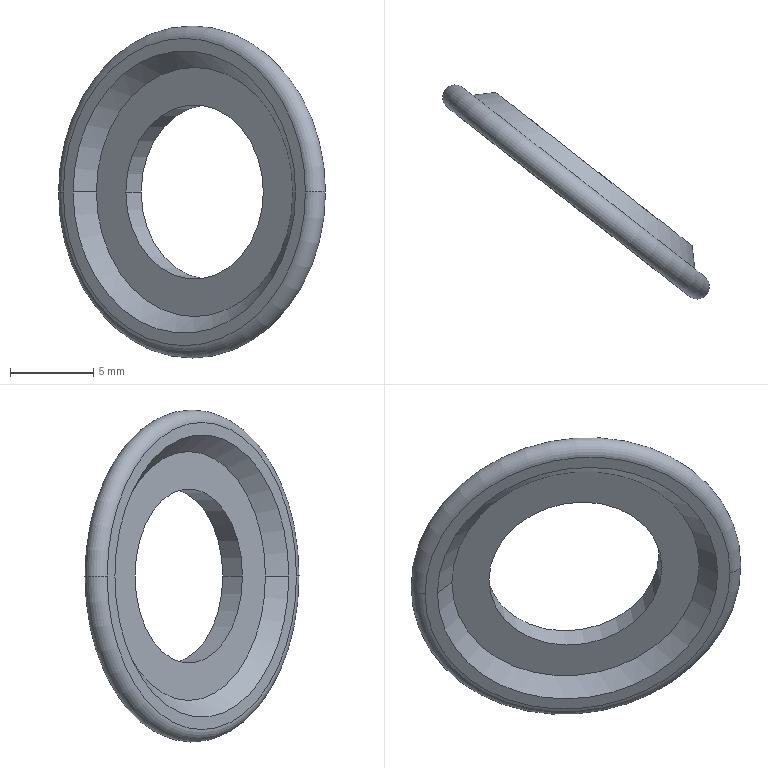Part | STEP file | VALVE_3PARTV11 | 1 solid | 12 faces | box 16.078 x 12.89 x 20 mm | volume 326.438 mm3 | cone 4 | plane 4 | torus 2 | cylinder 2 | commonest cylinder face diameters 10.5 x2
STEP:
#1=CARTESIAN_POINT('',(0.,0.,0.));
#2=DIRECTION('',(0.,0.,1.));
#3=DIRECTION('',(1.,0.,0.));
#4=AXIS2_PLACEMENT_3D('',#1,#2,#3);
#5=CARTESIAN_POINT('',(-0.6961,8.953,0.));
#6=VERTEX_POINT('',#5);
#7=CARTESIAN_POINT('',(13.882,-2.437,0.));
#8=VERTEX_POINT('',#7);
#9=CARTESIAN_POINT('',(6.593,3.258,0.));
#10=DIRECTION('',(0.6157,0.788,0.));
#11=DIRECTION('',(-0.788,0.6157,0.));
#12=AXIS2_PLACEMENT_3D('',#9,#10,#11);
#13=CIRCLE('',#12,9.25);
#14=CARTESIAN_POINT('',(7.055,3.849,0.));
#15=DIRECTION('',(0.6157,0.788,0.));
#16=DIRECTION('',(-0.788,0.6157,0.));
#17=AXIS2_PLACEMENT_3D('',#14,#15,#16);
#18=TOROIDAL_SURFACE('',#17,9.25,0.75);
#19=CARTESIAN_POINT('',(0.,-1.571));
#20=DIRECTION('',(1.,0.));
#21=VECTOR('',#20,1.);
#22=LINE('',#19,#21);
#23=(GEOMETRIC_REPRESENTATION_CONTEXT(2)PARAMETRIC_REPRESENTATION_CONTEXT()REPRESENTATION_CONTEXT('',''));
#24=DEFINITIONAL_REPRESENTATION('',(#22),#23);
#25=PCURVE('',#18,#24);
#26=CARTESIAN_POINT('',(-0.6961,8.953,0.));
#27=DIRECTION('',(-0.6157,-0.788,0.));
#28=DIRECTION('',(0.788,-0.6157,0.));
#29=AXIS2_PLACEMENT_3D('',#26,#27,#28);
#30=PLANE('',#29);
#31=CARTESIAN_POINT('',(0.,0.));
#32=CARTESIAN_POINT('',(0.,16.021));
#33=CARTESIAN_POINT('',(13.875,8.011));
#34=CARTESIAN_POINT('',(27.75,0.));
#35=CARTESIAN_POINT('',(13.875,-8.011));
#36=CARTESIAN_POINT('',(0.,-16.021));
#37=CARTESIAN_POINT('',(0.,0.));
#38=(BOUNDED_CURVE()B_SPLINE_CURVE(2,(#31,#32,#33,#34,#35,#36,#37),.UNSPECIFIED.,.T.,.F.)B_SPLINE_CURVE_WITH_KNOTS((1,2,2,2,2,1),(-2.094,0.,2.094,4.189,6.283,8.378),.UNSPECIFIED.)CURVE()GEOMETRIC_REPRESENTATION_ITEM()RATIONAL_B_SPLINE_CURVE((1.,0.5,1.,0.5,1.,0.5,1.))REPRESENTATION_ITEM(''));
#39=(GEOMETRIC_REPRESENTATION_CONTEXT(2)PARAMETRIC_REPRESENTATION_CONTEXT()REPRESENTATION_CONTEXT('',''));
#40=DEFINITIONAL_REPRESENTATION('',(#38),#39);
#41=PCURVE('',#30,#40);
#42=SURFACE_CURVE('',#13,(#25,#41),.PCURVE_S1.);
#43=EDGE_CURVE('',#6,#8,#42,.T.);
#44=ORIENTED_EDGE('',*,*,#43,.T.);
#45=CARTESIAN_POINT('',(14.806,-1.255,0.));
#46=VERTEX_POINT('',#45);
#47=CARTESIAN_POINT('',(14.344,-1.846,0.));
#48=DIRECTION('',(0.,0.,1.));
#49=DIRECTION('',(1.,0.,0.));
#50=AXIS2_PLACEMENT_3D('',#47,#48,#49);
#51=CIRCLE('',#50,0.75);
#52=CARTESIAN_POINT('',(3.142,-5.62));
#53=DIRECTION('',(0.,1.));
#54=VECTOR('',#53,1.);
#55=LINE('',#52,#54);
#56=(GEOMETRIC_REPRESENTATION_CONTEXT(2)PARAMETRIC_REPRESENTATION_CONTEXT()REPRESENTATION_CONTEXT('',''));
#57=DEFINITIONAL_REPRESENTATION('',(#55),#56);
#58=PCURVE('',#18,#57);
#59=CARTESIAN_POINT('',(7.055,3.849,0.));
#60=DIRECTION('',(0.6157,0.788,0.));
#61=DIRECTION('',(-0.788,0.6157,0.));
#62=AXIS2_PLACEMENT_3D('',#59,#60,#61);
#63=TOROIDAL_SURFACE('',#62,9.25,0.75);
#64=CARTESIAN_POINT('',(3.142,-5.62));
#65=DIRECTION('',(0.,1.));
#66=VECTOR('',#65,1.);
#67=LINE('',#64,#66);
#68=(GEOMETRIC_REPRESENTATION_CONTEXT(2)PARAMETRIC_REPRESENTATION_CONTEXT()REPRESENTATION_CONTEXT('',''));
#69=DEFINITIONAL_REPRESENTATION('',(#67),#68);
#70=PCURVE('',#63,#69);
#71=SURFACE_CURVE('',#51,(#58,#70),.PCURVE_S1.);
#72=EDGE_CURVE('',#8,#46,#71,.T.);
#73=ORIENTED_EDGE('',*,*,#72,.T.);
#74=CARTESIAN_POINT('',(0.2274,10.135,0.));
#75=VERTEX_POINT('',#74);
#76=CARTESIAN_POINT('',(7.517,4.44,0.));
#77=DIRECTION('',(0.6157,0.788,0.));
#78=DIRECTION('',(-0.788,0.6157,0.));
#79=AXIS2_PLACEMENT_3D('',#76,#77,#78);
#80=CIRCLE('',#79,9.25);
#81=CARTESIAN_POINT('',(0.,1.571));
#82=DIRECTION('',(1.,0.));
#83=VECTOR('',#82,1.);
#84=LINE('',#81,#83);
#85=(GEOMETRIC_REPRESENTATION_CONTEXT(2)PARAMETRIC_REPRESENTATION_CONTEXT()REPRESENTATION_CONTEXT('',''));
#86=DEFINITIONAL_REPRESENTATION('',(#84),#85);
#87=PCURVE('',#18,#86);
#88=CARTESIAN_POINT('',(0.8184,9.673,0.));
#89=DIRECTION('',(0.6157,0.788,0.));
#90=DIRECTION('',(-0.788,0.6157,0.));
#91=AXIS2_PLACEMENT_3D('',#88,#89,#90);
#92=PLANE('',#91);
#93=CARTESIAN_POINT('',(-8.5,0.));
#94=DIRECTION('',(1.,0.));
#95=AXIS2_PLACEMENT_2D('',#93,#94);
#96=CIRCLE('',#95,9.25);
#97=(GEOMETRIC_REPRESENTATION_CONTEXT(2)PARAMETRIC_REPRESENTATION_CONTEXT()REPRESENTATION_CONTEXT('',''));
#98=DEFINITIONAL_REPRESENTATION('',(#96),#97);
#99=PCURVE('',#92,#98);
#100=SURFACE_CURVE('',#80,(#87,#99),.PCURVE_S1.);
#101=EDGE_CURVE('',#75,#46,#100,.T.);
#102=ORIENTED_EDGE('',*,*,#101,.F.);
#103=CARTESIAN_POINT('',(-0.2343,9.544,0.));
#104=DIRECTION('',(0.,0.,-1.));
#105=DIRECTION('',(-1.,0.,0.));
#106=AXIS2_PLACEMENT_3D('',#103,#104,#105);
#107=CIRCLE('',#106,0.75);
#108=CARTESIAN_POINT('',(0.,-6.946));
#109=DIRECTION('',(0.,1.));
#110=VECTOR('',#109,1.);
#111=LINE('',#108,#110);
#112=(GEOMETRIC_REPRESENTATION_CONTEXT(2)PARAMETRIC_REPRESENTATION_CONTEXT()REPRESENTATION_CONTEXT('',''));
#113=DEFINITIONAL_REPRESENTATION('',(#111),#112);
#114=PCURVE('',#18,#113);
#115=CARTESIAN_POINT('',(6.283,-6.946));
#116=DIRECTION('',(0.,1.));
#117=VECTOR('',#116,1.);
#118=LINE('',#115,#117);
#119=(GEOMETRIC_REPRESENTATION_CONTEXT(2)PARAMETRIC_REPRESENTATION_CONTEXT()REPRESENTATION_CONTEXT('',''));
#120=DEFINITIONAL_REPRESENTATION('',(#118),#119);
#121=PCURVE('',#63,#120);
#122=SURFACE_CURVE('',#107,(#114,#121),.PCURVE_S1.);
#123=EDGE_CURVE('',#6,#75,#122,.T.);
#124=ORIENTED_EDGE('',*,*,#123,.F.);
#125=EDGE_LOOP('',(#44,#73,#102,#124));
#126=FACE_BOUND('',#125,.T.);
#127=ADVANCED_FACE('',(#126),#18,.T.);
#128=CARTESIAN_POINT('',(2.222,9.846,0.));
#129=VERTEX_POINT('',#128);
#130=CARTESIAN_POINT('',(14.042,0.6108,0.));
#131=VERTEX_POINT('',#130);
#132=CARTESIAN_POINT('',(8.132,5.228,0.));
#133=DIRECTION('',(0.6157,0.788,0.));
#134=DIRECTION('',(-0.788,0.6157,0.));
#135=AXIS2_PLACEMENT_3D('',#132,#133,#134);
#136=CIRCLE('',#135,7.5);
#137=CARTESIAN_POINT('',(8.132,5.228,0.));
#138=DIRECTION('',(-0.6157,-0.788,0.));
#139=DIRECTION('',(0.788,-0.6157,0.));
#140=AXIS2_PLACEMENT_3D('',#137,#138,#139);
#141=CONICAL_SURFACE('',#140,7.5,0.7854);
#142=CARTESIAN_POINT('',(3.142,0.));
#143=DIRECTION('',(-1.,0.));
#144=VECTOR('',#143,1.);
#145=LINE('',#142,#144);
#146=(GEOMETRIC_REPRESENTATION_CONTEXT(2)PARAMETRIC_REPRESENTATION_CONTEXT()REPRESENTATION_CONTEXT('',''));
#147=DEFINITIONAL_REPRESENTATION('',(#145),#146);
#148=PCURVE('',#141,#147);
#149=CARTESIAN_POINT('',(3.995,8.46,0.));
#150=DIRECTION('',(0.6157,0.788,0.));
#151=DIRECTION('',(-0.788,0.6157,0.));
#152=AXIS2_PLACEMENT_3D('',#149,#150,#151);
#153=PLANE('',#152);
#154=CARTESIAN_POINT('',(-5.25,0.));
#155=DIRECTION('',(1.,0.));
#156=AXIS2_PLACEMENT_2D('',#154,#155);
#157=CIRCLE('',#156,7.5);
#158=(GEOMETRIC_REPRESENTATION_CONTEXT(2)PARAMETRIC_REPRESENTATION_CONTEXT()REPRESENTATION_CONTEXT('',''));
#159=DEFINITIONAL_REPRESENTATION('',(#157),#158);
#160=PCURVE('',#153,#159);
#161=SURFACE_CURVE('',#136,(#148,#160),.PCURVE_S1.);
#162=EDGE_CURVE('',#129,#131,#161,.T.);
#163=ORIENTED_EDGE('',*,*,#162,.F.);
#164=CARTESIAN_POINT('',(0.8184,9.673,0.));
#165=VERTEX_POINT('',#164);
#166=CARTESIAN_POINT('',(2.222,9.846,0.));
#167=DIRECTION('',(-0.9925,-0.1219,0.));
#168=VECTOR('',#167,1.);
#169=LINE('',#166,#168);
#170=CARTESIAN_POINT('',(3.142,0.));
#171=DIRECTION('',(0.,1.));
#172=VECTOR('',#171,1.);
#173=LINE('',#170,#172);
#174=(GEOMETRIC_REPRESENTATION_CONTEXT(2)PARAMETRIC_REPRESENTATION_CONTEXT()REPRESENTATION_CONTEXT('',''));
#175=DEFINITIONAL_REPRESENTATION('',(#173),#174);
#176=PCURVE('',#141,#175);
#177=CARTESIAN_POINT('',(8.132,5.228,0.));
#178=DIRECTION('',(-0.6157,-0.788,0.));
#179=DIRECTION('',(0.788,-0.6157,0.));
#180=AXIS2_PLACEMENT_3D('',#177,#178,#179);
#181=CONICAL_SURFACE('',#180,7.5,0.7854);
#182=CARTESIAN_POINT('',(3.142,0.));
#183=DIRECTION('',(0.,1.));
#184=VECTOR('',#183,1.);
#185=LINE('',#182,#184);
#186=(GEOMETRIC_REPRESENTATION_CONTEXT(2)PARAMETRIC_REPRESENTATION_CONTEXT()REPRESENTATION_CONTEXT('',''));
#187=DEFINITIONAL_REPRESENTATION('',(#185),#186);
#188=PCURVE('',#181,#187);
#189=SURFACE_CURVE('',#169,(#176,#188),.PCURVE_S1.);
#190=EDGE_CURVE('',#129,#165,#189,.T.);
#191=ORIENTED_EDGE('',*,*,#190,.T.);
#192=CARTESIAN_POINT('',(14.215,-0.7929,0.));
#193=VERTEX_POINT('',#192);
#194=CARTESIAN_POINT('',(7.517,4.44,0.));
#195=DIRECTION('',(0.6157,0.788,0.));
#196=DIRECTION('',(-0.788,0.6157,0.));
#197=AXIS2_PLACEMENT_3D('',#194,#195,#196);
#198=CIRCLE('',#197,8.5);
#199=CARTESIAN_POINT('',(3.142,1.));
#200=DIRECTION('',(-1.,0.));
#201=VECTOR('',#200,1.);
#202=LINE('',#199,#201);
#203=(GEOMETRIC_REPRESENTATION_CONTEXT(2)PARAMETRIC_REPRESENTATION_CONTEXT()REPRESENTATION_CONTEXT('',''));
#204=DEFINITIONAL_REPRESENTATION('',(#202),#203);
#205=PCURVE('',#141,#204);
#206=CARTESIAN_POINT('',(-8.5,0.));
#207=DIRECTION('',(1.,0.));
#208=AXIS2_PLACEMENT_2D('',#206,#207);
#209=CIRCLE('',#208,8.5);
#210=(GEOMETRIC_REPRESENTATION_CONTEXT(2)PARAMETRIC_REPRESENTATION_CONTEXT()REPRESENTATION_CONTEXT('',''));
#211=DEFINITIONAL_REPRESENTATION('',(#209),#210);
#212=PCURVE('',#92,#211);
#213=SURFACE_CURVE('',#198,(#205,#212),.PCURVE_S1.);
#214=EDGE_CURVE('',#165,#193,#213,.T.);
#215=ORIENTED_EDGE('',*,*,#214,.T.);
#216=CARTESIAN_POINT('',(14.042,0.6108,0.));
#217=DIRECTION('',(0.1219,-0.9925,0.));
#218=VECTOR('',#217,1.);
#219=LINE('',#216,#218);
#220=CARTESIAN_POINT('',(0.,0.));
#221=DIRECTION('',(0.,1.));
#222=VECTOR('',#221,1.);
#223=LINE('',#220,#222);
#224=(GEOMETRIC_REPRESENTATION_CONTEXT(2)PARAMETRIC_REPRESENTATION_CONTEXT()REPRESENTATION_CONTEXT('',''));
#225=DEFINITIONAL_REPRESENTATION('',(#223),#224);
#226=PCURVE('',#141,#225);
#227=CARTESIAN_POINT('',(6.283,0.));
#228=DIRECTION('',(0.,1.));
#229=VECTOR('',#228,1.);
#230=LINE('',#227,#229);
#231=(GEOMETRIC_REPRESENTATION_CONTEXT(2)PARAMETRIC_REPRESENTATION_CONTEXT()REPRESENTATION_CONTEXT('',''));
#232=DEFINITIONAL_REPRESENTATION('',(#230),#231);
#233=PCURVE('',#181,#232);
#234=SURFACE_CURVE('',#219,(#226,#233),.PCURVE_S1.);
#235=EDGE_CURVE('',#131,#193,#234,.T.);
#236=ORIENTED_EDGE('',*,*,#235,.F.);
#237=EDGE_LOOP('',(#163,#191,#215,#236));
#238=FACE_BOUND('',#237,.T.);
#239=ADVANCED_FACE('',(#238),#141,.T.);
#240=CARTESIAN_POINT('',(3.072,7.278,0.));
#241=VERTEX_POINT('',#240);
#242=CARTESIAN_POINT('',(3.995,8.46,0.));
#243=VERTEX_POINT('',#242);
#244=CARTESIAN_POINT('',(-6.471,-4.936,0.));
#245=DIRECTION('',(0.6157,0.788,0.));
#246=VECTOR('',#245,1.);
#247=LINE('',#244,#246);
#248=CARTESIAN_POINT('',(-2.334,-8.168,0.));
#249=DIRECTION('',(0.6157,0.788,0.));
#250=DIRECTION('',(-0.788,0.6157,0.));
#251=AXIS2_PLACEMENT_3D('',#248,#249,#250);
#252=CYLINDRICAL_SURFACE('',#251,5.25);
#253=CARTESIAN_POINT('',(6.283,0.));
#254=DIRECTION('',(0.,1.));
#255=VECTOR('',#254,1.);
#256=LINE('',#253,#255);
#257=(GEOMETRIC_REPRESENTATION_CONTEXT(2)PARAMETRIC_REPRESENTATION_CONTEXT()REPRESENTATION_CONTEXT('',''));
#258=DEFINITIONAL_REPRESENTATION('',(#256),#257);
#259=PCURVE('',#252,#258);
#260=CARTESIAN_POINT('',(-2.334,-8.168,0.));
#261=DIRECTION('',(0.6157,0.788,0.));
#262=DIRECTION('',(-0.788,0.6157,0.));
#263=AXIS2_PLACEMENT_3D('',#260,#261,#262);
#264=CYLINDRICAL_SURFACE('',#263,5.25);
#265=CARTESIAN_POINT('',(0.,0.));
#266=DIRECTION('',(0.,1.));
#267=VECTOR('',#266,1.);
#268=LINE('',#265,#267);
#269=(GEOMETRIC_REPRESENTATION_CONTEXT(2)PARAMETRIC_REPRESENTATION_CONTEXT()REPRESENTATION_CONTEXT('',''));
#270=DEFINITIONAL_REPRESENTATION('',(#268),#269);
#271=PCURVE('',#264,#270);
#272=SURFACE_CURVE('',#247,(#259,#271),.PCURVE_S1.);
#273=EDGE_CURVE('',#241,#243,#272,.T.);
#274=ORIENTED_EDGE('',*,*,#273,.T.);
#275=CARTESIAN_POINT('',(12.269,1.996,0.));
#276=VERTEX_POINT('',#275);
#277=CARTESIAN_POINT('',(8.132,5.228,0.));
#278=DIRECTION('',(0.6157,0.788,0.));
#279=DIRECTION('',(-0.788,0.6157,0.));
#280=AXIS2_PLACEMENT_3D('',#277,#278,#279);
#281=CIRCLE('',#280,5.25);
#282=CARTESIAN_POINT('',(0.,17.));
#283=DIRECTION('',(1.,0.));
#284=VECTOR('',#283,1.);
#285=LINE('',#282,#284);
#286=(GEOMETRIC_REPRESENTATION_CONTEXT(2)PARAMETRIC_REPRESENTATION_CONTEXT()REPRESENTATION_CONTEXT('',''));
#287=DEFINITIONAL_REPRESENTATION('',(#285),#286);
#288=PCURVE('',#252,#287);
#289=CARTESIAN_POINT('',(-5.25,0.));
#290=DIRECTION('',(1.,0.));
#291=AXIS2_PLACEMENT_2D('',#289,#290);
#292=CIRCLE('',#291,5.25);
#293=(GEOMETRIC_REPRESENTATION_CONTEXT(2)PARAMETRIC_REPRESENTATION_CONTEXT()REPRESENTATION_CONTEXT('',''));
#294=DEFINITIONAL_REPRESENTATION('',(#292),#293);
#295=PCURVE('',#153,#294);
#296=SURFACE_CURVE('',#281,(#288,#295),.PCURVE_S1.);
#297=EDGE_CURVE('',#276,#243,#296,.T.);
#298=ORIENTED_EDGE('',*,*,#297,.F.);
#299=CARTESIAN_POINT('',(11.346,0.814,0.));
#300=VERTEX_POINT('',#299);
#301=CARTESIAN_POINT('',(1.803,-11.4,0.));
#302=DIRECTION('',(0.6157,0.788,0.));
#303=VECTOR('',#302,1.);
#304=LINE('',#301,#303);
#305=CARTESIAN_POINT('',(3.142,0.));
#306=DIRECTION('',(0.,1.));
#307=VECTOR('',#306,1.);
#308=LINE('',#305,#307);
#309=(GEOMETRIC_REPRESENTATION_CONTEXT(2)PARAMETRIC_REPRESENTATION_CONTEXT()REPRESENTATION_CONTEXT('',''));
#310=DEFINITIONAL_REPRESENTATION('',(#308),#309);
#311=PCURVE('',#252,#310);
#312=CARTESIAN_POINT('',(3.142,0.));
#313=DIRECTION('',(0.,1.));
#314=VECTOR('',#313,1.);
#315=LINE('',#312,#314);
#316=(GEOMETRIC_REPRESENTATION_CONTEXT(2)PARAMETRIC_REPRESENTATION_CONTEXT()REPRESENTATION_CONTEXT('',''));
#317=DEFINITIONAL_REPRESENTATION('',(#315),#316);
#318=PCURVE('',#264,#317);
#319=SURFACE_CURVE('',#304,(#311,#318),.PCURVE_S1.);
#320=EDGE_CURVE('',#300,#276,#319,.T.);
#321=ORIENTED_EDGE('',*,*,#320,.F.);
#322=CARTESIAN_POINT('',(7.209,4.046,0.));
#323=DIRECTION('',(0.6157,0.788,0.));
#324=DIRECTION('',(-0.788,0.6157,0.));
#325=AXIS2_PLACEMENT_3D('',#322,#323,#324);
#326=CIRCLE('',#325,5.25);
#327=CARTESIAN_POINT('',(0.,15.5));
#328=DIRECTION('',(1.,0.));
#329=VECTOR('',#328,1.);
#330=LINE('',#327,#329);
#331=(GEOMETRIC_REPRESENTATION_CONTEXT(2)PARAMETRIC_REPRESENTATION_CONTEXT()REPRESENTATION_CONTEXT('',''));
#332=DEFINITIONAL_REPRESENTATION('',(#330),#331);
#333=PCURVE('',#252,#332);
#334=CARTESIAN_POINT('',(1.299,8.664,0.));
#335=DIRECTION('',(-0.6157,-0.788,0.));
#336=DIRECTION('',(0.788,-0.6157,0.));
#337=AXIS2_PLACEMENT_3D('',#334,#335,#336);
#338=PLANE('',#337);
#339=CARTESIAN_POINT('',(2.25,0.));
#340=CARTESIAN_POINT('',(2.25,9.093));
#341=CARTESIAN_POINT('',(10.125,4.547));
#342=CARTESIAN_POINT('',(18.,0.));
#343=CARTESIAN_POINT('',(10.125,-4.547));
#344=CARTESIAN_POINT('',(2.25,-9.093));
#345=CARTESIAN_POINT('',(2.25,0.));
#346=(BOUNDED_CURVE()B_SPLINE_CURVE(2,(#339,#340,#341,#342,#343,#344,#345),.UNSPECIFIED.,.T.,.F.)B_SPLINE_CURVE_WITH_KNOTS((1,2,2,2,2,1),(-2.094,0.,2.094,4.189,6.283,8.378),.UNSPECIFIED.)CURVE()GEOMETRIC_REPRESENTATION_ITEM()RATIONAL_B_SPLINE_CURVE((1.,0.5,1.,0.5,1.,0.5,1.))REPRESENTATION_ITEM(''));
#347=(GEOMETRIC_REPRESENTATION_CONTEXT(2)PARAMETRIC_REPRESENTATION_CONTEXT()REPRESENTATION_CONTEXT('',''));
#348=DEFINITIONAL_REPRESENTATION('',(#346),#347);
#349=PCURVE('',#338,#348);
#350=SURFACE_CURVE('',#326,(#333,#349),.PCURVE_S1.);
#351=EDGE_CURVE('',#300,#241,#350,.T.);
#352=ORIENTED_EDGE('',*,*,#351,.T.);
#353=EDGE_LOOP('',(#274,#298,#321,#352));
#354=FACE_BOUND('',#353,.F.);
#355=ADVANCED_FACE('',(#354),#252,.F.);
#356=CARTESIAN_POINT('',(13.119,-0.5713,0.));
#357=VERTEX_POINT('',#356);
#358=CARTESIAN_POINT('',(13.291,-1.975,0.));
#359=VERTEX_POINT('',#358);
#360=CARTESIAN_POINT('',(13.291,-1.975,0.));
#361=DIRECTION('',(0.1219,-0.9925,0.));
#362=VECTOR('',#361,1.);
#363=LINE('',#360,#362);
#364=CARTESIAN_POINT('',(6.593,3.258,0.));
#365=DIRECTION('',(-0.6157,-0.788,0.));
#366=DIRECTION('',(0.788,-0.6157,0.));
#367=AXIS2_PLACEMENT_3D('',#364,#365,#366);
#368=CONICAL_SURFACE('',#367,8.5,0.7854);
#369=CARTESIAN_POINT('',(6.283,0.));
#370=DIRECTION('',(0.,1.));
#371=VECTOR('',#370,1.);
#372=LINE('',#369,#371);
#373=(GEOMETRIC_REPRESENTATION_CONTEXT(2)PARAMETRIC_REPRESENTATION_CONTEXT()REPRESENTATION_CONTEXT('',''));
#374=DEFINITIONAL_REPRESENTATION('',(#372),#373);
#375=PCURVE('',#368,#374);
#376=CARTESIAN_POINT('',(6.593,3.258,0.));
#377=DIRECTION('',(-0.6157,-0.788,0.));
#378=DIRECTION('',(0.788,-0.6157,0.));
#379=AXIS2_PLACEMENT_3D('',#376,#377,#378);
#380=CONICAL_SURFACE('',#379,8.5,0.7854);
#381=CARTESIAN_POINT('',(0.,0.));
#382=DIRECTION('',(0.,1.));
#383=VECTOR('',#382,1.);
#384=LINE('',#381,#383);
#385=(GEOMETRIC_REPRESENTATION_CONTEXT(2)PARAMETRIC_REPRESENTATION_CONTEXT()REPRESENTATION_CONTEXT('',''));
#386=DEFINITIONAL_REPRESENTATION('',(#384),#385);
#387=PCURVE('',#380,#386);
#388=SURFACE_CURVE('',#363,(#375,#387),.PCURVE_S1.);
#389=EDGE_CURVE('',#357,#359,#388,.T.);
#390=ORIENTED_EDGE('',*,*,#389,.T.);
#391=CARTESIAN_POINT('',(-0.105,8.491,0.));
#392=VERTEX_POINT('',#391);
#393=CARTESIAN_POINT('',(6.593,3.258,0.));
#394=DIRECTION('',(0.6157,0.788,0.));
#395=DIRECTION('',(-0.788,0.6157,0.));
#396=AXIS2_PLACEMENT_3D('',#393,#394,#395);
#397=CIRCLE('',#396,8.5);
#398=CARTESIAN_POINT('',(9.425,0.));
#399=DIRECTION('',(-1.,0.));
#400=VECTOR('',#399,1.);
#401=LINE('',#398,#400);
#402=(GEOMETRIC_REPRESENTATION_CONTEXT(2)PARAMETRIC_REPRESENTATION_CONTEXT()REPRESENTATION_CONTEXT('',''));
#403=DEFINITIONAL_REPRESENTATION('',(#401),#402);
#404=PCURVE('',#368,#403);
#405=CARTESIAN_POINT('',(0.75,0.));
#406=CARTESIAN_POINT('',(0.75,14.722));
#407=CARTESIAN_POINT('',(13.5,7.361));
#408=CARTESIAN_POINT('',(26.25,0.));
#409=CARTESIAN_POINT('',(13.5,-7.361));
#410=CARTESIAN_POINT('',(0.75,-14.722));
#411=CARTESIAN_POINT('',(0.75,0.));
#412=(BOUNDED_CURVE()B_SPLINE_CURVE(2,(#405,#406,#407,#408,#409,#410,#411),.UNSPECIFIED.,.T.,.F.)B_SPLINE_CURVE_WITH_KNOTS((1,2,2,2,2,1),(-2.094,0.,2.094,4.189,6.283,8.378),.UNSPECIFIED.)CURVE()GEOMETRIC_REPRESENTATION_ITEM()RATIONAL_B_SPLINE_CURVE((1.,0.5,1.,0.5,1.,0.5,1.))REPRESENTATION_ITEM(''));
#413=(GEOMETRIC_REPRESENTATION_CONTEXT(2)PARAMETRIC_REPRESENTATION_CONTEXT()REPRESENTATION_CONTEXT('',''));
#414=DEFINITIONAL_REPRESENTATION('',(#412),#413);
#415=PCURVE('',#30,#414);
#416=SURFACE_CURVE('',#397,(#404,#415),.PCURVE_S1.);
#417=EDGE_CURVE('',#359,#392,#416,.T.);
#418=ORIENTED_EDGE('',*,*,#417,.T.);
#419=CARTESIAN_POINT('',(1.299,8.664,0.));
#420=VERTEX_POINT('',#419);
#421=CARTESIAN_POINT('',(-0.105,8.491,0.));
#422=DIRECTION('',(-0.9925,-0.1219,0.));
#423=VECTOR('',#422,1.);
#424=LINE('',#421,#423);
#425=CARTESIAN_POINT('',(3.142,0.));
#426=DIRECTION('',(0.,1.));
#427=VECTOR('',#426,1.);
#428=LINE('',#425,#427);
#429=(GEOMETRIC_REPRESENTATION_CONTEXT(2)PARAMETRIC_REPRESENTATION_CONTEXT()REPRESENTATION_CONTEXT('',''));
#430=DEFINITIONAL_REPRESENTATION('',(#428),#429);
#431=PCURVE('',#368,#430);
#432=CARTESIAN_POINT('',(3.142,0.));
#433=DIRECTION('',(0.,1.));
#434=VECTOR('',#433,1.);
#435=LINE('',#432,#434);
#436=(GEOMETRIC_REPRESENTATION_CONTEXT(2)PARAMETRIC_REPRESENTATION_CONTEXT()REPRESENTATION_CONTEXT('',''));
#437=DEFINITIONAL_REPRESENTATION('',(#435),#436);
#438=PCURVE('',#380,#437);
#439=SURFACE_CURVE('',#424,(#431,#438),.PCURVE_S1.);
#440=EDGE_CURVE('',#420,#392,#439,.T.);
#441=ORIENTED_EDGE('',*,*,#440,.F.);
#442=CARTESIAN_POINT('',(7.209,4.046,0.));
#443=DIRECTION('',(0.6157,0.788,0.));
#444=DIRECTION('',(-0.788,0.6157,0.));
#445=AXIS2_PLACEMENT_3D('',#442,#443,#444);
#446=CIRCLE('',#445,7.5);
#447=CARTESIAN_POINT('',(9.425,-1.));
#448=DIRECTION('',(-1.,0.));
#449=VECTOR('',#448,1.);
#450=LINE('',#447,#449);
#451=(GEOMETRIC_REPRESENTATION_CONTEXT(2)PARAMETRIC_REPRESENTATION_CONTEXT()REPRESENTATION_CONTEXT('',''));
#452=DEFINITIONAL_REPRESENTATION('',(#450),#451);
#453=PCURVE('',#368,#452);
#454=CARTESIAN_POINT('',(0.,0.));
#455=CARTESIAN_POINT('',(0.,12.99));
#456=CARTESIAN_POINT('',(11.25,6.495));
#457=CARTESIAN_POINT('',(22.5,0.));
#458=CARTESIAN_POINT('',(11.25,-6.495));
#459=CARTESIAN_POINT('',(0.,-12.99));
#460=CARTESIAN_POINT('',(0.,0.));
#461=(BOUNDED_CURVE()B_SPLINE_CURVE(2,(#454,#455,#456,#457,#458,#459,#460),.UNSPECIFIED.,.T.,.F.)B_SPLINE_CURVE_WITH_KNOTS((1,2,2,2,2,1),(-2.094,0.,2.094,4.189,6.283,8.378),.UNSPECIFIED.)CURVE()GEOMETRIC_REPRESENTATION_ITEM()RATIONAL_B_SPLINE_CURVE((1.,0.5,1.,0.5,1.,0.5,1.))REPRESENTATION_ITEM(''));
#462=(GEOMETRIC_REPRESENTATION_CONTEXT(2)PARAMETRIC_REPRESENTATION_CONTEXT()REPRESENTATION_CONTEXT('',''));
#463=DEFINITIONAL_REPRESENTATION('',(#461),#462);
#464=PCURVE('',#338,#463);
#465=SURFACE_CURVE('',#446,(#453,#464),.PCURVE_S1.);
#466=EDGE_CURVE('',#357,#420,#465,.T.);
#467=ORIENTED_EDGE('',*,*,#466,.F.);
#468=EDGE_LOOP('',(#390,#418,#441,#467));
#469=FACE_BOUND('',#468,.F.);
#470=ADVANCED_FACE('',(#469),#368,.F.);
#471=CARTESIAN_POINT('',(6.593,3.258,0.));
#472=DIRECTION('',(0.6157,0.788,0.));
#473=DIRECTION('',(-0.788,0.6157,0.));
#474=AXIS2_PLACEMENT_3D('',#471,#472,#473);
#475=CIRCLE('',#474,8.5);
#476=CARTESIAN_POINT('',(3.142,0.));
#477=DIRECTION('',(-1.,0.));
#478=VECTOR('',#477,1.);
#479=LINE('',#476,#478);
#480=(GEOMETRIC_REPRESENTATION_CONTEXT(2)PARAMETRIC_REPRESENTATION_CONTEXT()REPRESENTATION_CONTEXT('',''));
#481=DEFINITIONAL_REPRESENTATION('',(#479),#480);
#482=PCURVE('',#380,#481);
#483=CARTESIAN_POINT('',(0.75,0.));
#484=CARTESIAN_POINT('',(0.75,14.722));
#485=CARTESIAN_POINT('',(13.5,7.361));
#486=CARTESIAN_POINT('',(26.25,0.));
#487=CARTESIAN_POINT('',(13.5,-7.361));
#488=CARTESIAN_POINT('',(0.75,-14.722));
#489=CARTESIAN_POINT('',(0.75,0.));
#490=(BOUNDED_CURVE()B_SPLINE_CURVE(2,(#483,#484,#485,#486,#487,#488,#489),.UNSPECIFIED.,.T.,.F.)B_SPLINE_CURVE_WITH_KNOTS((1,2,2,2,2,1),(-2.094,0.,2.094,4.189,6.283,8.378),.UNSPECIFIED.)CURVE()GEOMETRIC_REPRESENTATION_ITEM()RATIONAL_B_SPLINE_CURVE((1.,0.5,1.,0.5,1.,0.5,1.))REPRESENTATION_ITEM(''));
#491=(GEOMETRIC_REPRESENTATION_CONTEXT(2)PARAMETRIC_REPRESENTATION_CONTEXT()REPRESENTATION_CONTEXT('',''));
#492=DEFINITIONAL_REPRESENTATION('',(#490),#491);
#493=PCURVE('',#30,#492);
#494=SURFACE_CURVE('',#475,(#482,#493),.PCURVE_S1.);
#495=EDGE_CURVE('',#392,#359,#494,.T.);
#496=ORIENTED_EDGE('',*,*,#495,.T.);
#497=ORIENTED_EDGE('',*,*,#389,.F.);
#498=CARTESIAN_POINT('',(7.209,4.046,0.));
#499=DIRECTION('',(0.6157,0.788,0.));
#500=DIRECTION('',(-0.788,0.6157,0.));
#501=AXIS2_PLACEMENT_3D('',#498,#499,#500);
#502=CIRCLE('',#501,7.5);
#503=CARTESIAN_POINT('',(3.142,-1.));
#504=DIRECTION('',(-1.,0.));
#505=VECTOR('',#504,1.);
#506=LINE('',#503,#505);
#507=(GEOMETRIC_REPRESENTATION_CONTEXT(2)PARAMETRIC_REPRESENTATION_CONTEXT()REPRESENTATION_CONTEXT('',''));
#508=DEFINITIONAL_REPRESENTATION('',(#506),#507);
#509=PCURVE('',#380,#508);
#510=CARTESIAN_POINT('',(0.,0.));
#511=CARTESIAN_POINT('',(0.,12.99));
#512=CARTESIAN_POINT('',(11.25,6.495));
#513=CARTESIAN_POINT('',(22.5,0.));
#514=CARTESIAN_POINT('',(11.25,-6.495));
#515=CARTESIAN_POINT('',(0.,-12.99));
#516=CARTESIAN_POINT('',(0.,0.));
#517=(BOUNDED_CURVE()B_SPLINE_CURVE(2,(#510,#511,#512,#513,#514,#515,#516),.UNSPECIFIED.,.T.,.F.)B_SPLINE_CURVE_WITH_KNOTS((1,2,2,2,2,1),(-2.094,0.,2.094,4.189,6.283,8.378),.UNSPECIFIED.)CURVE()GEOMETRIC_REPRESENTATION_ITEM()RATIONAL_B_SPLINE_CURVE((1.,0.5,1.,0.5,1.,0.5,1.))REPRESENTATION_ITEM(''));
#518=(GEOMETRIC_REPRESENTATION_CONTEXT(2)PARAMETRIC_REPRESENTATION_CONTEXT()REPRESENTATION_CONTEXT('',''));
#519=DEFINITIONAL_REPRESENTATION('',(#517),#518);
#520=PCURVE('',#338,#519);
#521=SURFACE_CURVE('',#502,(#509,#520),.PCURVE_S1.);
#522=EDGE_CURVE('',#420,#357,#521,.T.);
#523=ORIENTED_EDGE('',*,*,#522,.F.);
#524=ORIENTED_EDGE('',*,*,#440,.T.);
#525=EDGE_LOOP('',(#496,#497,#523,#524));
#526=FACE_BOUND('',#525,.F.);
#527=ADVANCED_FACE('',(#526),#380,.F.);
#528=CARTESIAN_POINT('',(7.209,4.046,0.));
#529=DIRECTION('',(0.6157,0.788,0.));
#530=DIRECTION('',(-0.788,0.6157,0.));
#531=AXIS2_PLACEMENT_3D('',#528,#529,#530);
#532=CIRCLE('',#531,5.25);
#533=CARTESIAN_POINT('',(2.25,0.));
#534=CARTESIAN_POINT('',(2.25,9.093));
#535=CARTESIAN_POINT('',(10.125,4.547));
#536=CARTESIAN_POINT('',(18.,0.));
#537=CARTESIAN_POINT('',(10.125,-4.547));
#538=CARTESIAN_POINT('',(2.25,-9.093));
#539=CARTESIAN_POINT('',(2.25,0.));
#540=(BOUNDED_CURVE()B_SPLINE_CURVE(2,(#533,#534,#535,#536,#537,#538,#539),.UNSPECIFIED.,.T.,.F.)B_SPLINE_CURVE_WITH_KNOTS((1,2,2,2,2,1),(-2.094,0.,2.094,4.189,6.283,8.378),.UNSPECIFIED.)CURVE()GEOMETRIC_REPRESENTATION_ITEM()RATIONAL_B_SPLINE_CURVE((1.,0.5,1.,0.5,1.,0.5,1.))REPRESENTATION_ITEM(''));
#541=(GEOMETRIC_REPRESENTATION_CONTEXT(2)PARAMETRIC_REPRESENTATION_CONTEXT()REPRESENTATION_CONTEXT('',''));
#542=DEFINITIONAL_REPRESENTATION('',(#540),#541);
#543=PCURVE('',#338,#542);
#544=CARTESIAN_POINT('',(0.,15.5));
#545=DIRECTION('',(1.,0.));
#546=VECTOR('',#545,1.);
#547=LINE('',#544,#546);
#548=(GEOMETRIC_REPRESENTATION_CONTEXT(2)PARAMETRIC_REPRESENTATION_CONTEXT()REPRESENTATION_CONTEXT('',''));
#549=DEFINITIONAL_REPRESENTATION('',(#547),#548);
#550=PCURVE('',#264,#549);
#551=SURFACE_CURVE('',#532,(#543,#550),.PCURVE_S1.);
#552=EDGE_CURVE('',#241,#300,#551,.T.);
#553=ORIENTED_EDGE('',*,*,#552,.T.);
#554=ORIENTED_EDGE('',*,*,#351,.T.);
#555=EDGE_LOOP('',(#553,#554));
#556=FACE_BOUND('',#555,.T.);
#557=ORIENTED_EDGE('',*,*,#466,.F.);
#558=ORIENTED_EDGE('',*,*,#522,.F.);
#559=EDGE_LOOP('',(#557,#558));
#560=FACE_BOUND('',#559,.T.);
#561=ADVANCED_FACE('',(#556,#560),#338,.T.);
#562=CARTESIAN_POINT('',(8.132,5.228,0.));
#563=DIRECTION('',(0.6157,0.788,0.));
#564=DIRECTION('',(-0.788,0.6157,0.));
#565=AXIS2_PLACEMENT_3D('',#562,#563,#564);
#566=CIRCLE('',#565,5.25);
#567=CARTESIAN_POINT('',(0.,17.));
#568=DIRECTION('',(1.,0.));
#569=VECTOR('',#568,1.);
#570=LINE('',#567,#569);
#571=(GEOMETRIC_REPRESENTATION_CONTEXT(2)PARAMETRIC_REPRESENTATION_CONTEXT()REPRESENTATION_CONTEXT('',''));
#572=DEFINITIONAL_REPRESENTATION('',(#570),#571);
#573=PCURVE('',#264,#572);
#574=CARTESIAN_POINT('',(-5.25,0.));
#575=DIRECTION('',(1.,0.));
#576=AXIS2_PLACEMENT_2D('',#574,#575);
#577=CIRCLE('',#576,5.25);
#578=(GEOMETRIC_REPRESENTATION_CONTEXT(2)PARAMETRIC_REPRESENTATION_CONTEXT()REPRESENTATION_CONTEXT('',''));
#579=DEFINITIONAL_REPRESENTATION('',(#577),#578);
#580=PCURVE('',#153,#579);
#581=SURFACE_CURVE('',#566,(#573,#580),.PCURVE_S1.);
#582=EDGE_CURVE('',#243,#276,#581,.T.);
#583=ORIENTED_EDGE('',*,*,#582,.F.);
#584=ORIENTED_EDGE('',*,*,#273,.F.);
#585=ORIENTED_EDGE('',*,*,#552,.T.);
#586=ORIENTED_EDGE('',*,*,#320,.T.);
#587=EDGE_LOOP('',(#583,#584,#585,#586));
#588=FACE_BOUND('',#587,.F.);
#589=ADVANCED_FACE('',(#588),#264,.F.);
#590=CARTESIAN_POINT('',(8.132,5.228,0.));
#591=DIRECTION('',(0.6157,0.788,0.));
#592=DIRECTION('',(-0.788,0.6157,0.));
#593=AXIS2_PLACEMENT_3D('',#590,#591,#592);
#594=CIRCLE('',#593,7.5);
#595=CARTESIAN_POINT('',(-5.25,0.));
#596=DIRECTION('',(1.,0.));
#597=AXIS2_PLACEMENT_2D('',#595,#596);
#598=CIRCLE('',#597,7.5);
#599=(GEOMETRIC_REPRESENTATION_CONTEXT(2)PARAMETRIC_REPRESENTATION_CONTEXT()REPRESENTATION_CONTEXT('',''));
#600=DEFINITIONAL_REPRESENTATION('',(#598),#599);
#601=PCURVE('',#153,#600);
#602=CARTESIAN_POINT('',(9.425,0.));
#603=DIRECTION('',(-1.,0.));
#604=VECTOR('',#603,1.);
#605=LINE('',#602,#604);
#606=(GEOMETRIC_REPRESENTATION_CONTEXT(2)PARAMETRIC_REPRESENTATION_CONTEXT()REPRESENTATION_CONTEXT('',''));
#607=DEFINITIONAL_REPRESENTATION('',(#605),#606);
#608=PCURVE('',#181,#607);
#609=SURFACE_CURVE('',#594,(#601,#608),.PCURVE_S1.);
#610=EDGE_CURVE('',#131,#129,#609,.T.);
#611=ORIENTED_EDGE('',*,*,#610,.T.);
#612=ORIENTED_EDGE('',*,*,#162,.T.);
#613=EDGE_LOOP('',(#611,#612));
#614=FACE_BOUND('',#613,.T.);
#615=ORIENTED_EDGE('',*,*,#582,.F.);
#616=ORIENTED_EDGE('',*,*,#297,.F.);
#617=EDGE_LOOP('',(#615,#616));
#618=FACE_BOUND('',#617,.T.);
#619=ADVANCED_FACE('',(#614,#618),#153,.T.);
#620=ORIENTED_EDGE('',*,*,#190,.F.);
#621=ORIENTED_EDGE('',*,*,#610,.F.);
#622=ORIENTED_EDGE('',*,*,#235,.T.);
#623=CARTESIAN_POINT('',(7.517,4.44,0.));
#624=DIRECTION('',(0.6157,0.788,0.));
#625=DIRECTION('',(-0.788,0.6157,0.));
#626=AXIS2_PLACEMENT_3D('',#623,#624,#625);
#627=CIRCLE('',#626,8.5);
#628=CARTESIAN_POINT('',(9.425,1.));
#629=DIRECTION('',(-1.,0.));
#630=VECTOR('',#629,1.);
#631=LINE('',#628,#630);
#632=(GEOMETRIC_REPRESENTATION_CONTEXT(2)PARAMETRIC_REPRESENTATION_CONTEXT()REPRESENTATION_CONTEXT('',''));
#633=DEFINITIONAL_REPRESENTATION('',(#631),#632);
#634=PCURVE('',#181,#633);
#635=CARTESIAN_POINT('',(-8.5,0.));
#636=DIRECTION('',(1.,0.));
#637=AXIS2_PLACEMENT_2D('',#635,#636);
#638=CIRCLE('',#637,8.5);
#639=(GEOMETRIC_REPRESENTATION_CONTEXT(2)PARAMETRIC_REPRESENTATION_CONTEXT()REPRESENTATION_CONTEXT('',''));
#640=DEFINITIONAL_REPRESENTATION('',(#638),#639);
#641=PCURVE('',#92,#640);
#642=SURFACE_CURVE('',#627,(#634,#641),.PCURVE_S1.);
#643=EDGE_CURVE('',#193,#165,#642,.T.);
#644=ORIENTED_EDGE('',*,*,#643,.T.);
#645=EDGE_LOOP('',(#620,#621,#622,#644));
#646=FACE_BOUND('',#645,.T.);
#647=ADVANCED_FACE('',(#646),#181,.T.);
#648=ORIENTED_EDGE('',*,*,#101,.T.);
#649=CARTESIAN_POINT('',(7.517,4.44,0.));
#650=DIRECTION('',(0.6157,0.788,0.));
#651=DIRECTION('',(-0.788,0.6157,0.));
#652=AXIS2_PLACEMENT_3D('',#649,#650,#651);
#653=CIRCLE('',#652,9.25);
#654=CARTESIAN_POINT('',(-8.5,0.));
#655=DIRECTION('',(1.,0.));
#656=AXIS2_PLACEMENT_2D('',#654,#655);
#657=CIRCLE('',#656,9.25);
#658=(GEOMETRIC_REPRESENTATION_CONTEXT(2)PARAMETRIC_REPRESENTATION_CONTEXT()REPRESENTATION_CONTEXT('',''));
#659=DEFINITIONAL_REPRESENTATION('',(#657),#658);
#660=PCURVE('',#92,#659);
#661=CARTESIAN_POINT('',(0.,1.571));
#662=DIRECTION('',(1.,0.));
#663=VECTOR('',#662,1.);
#664=LINE('',#661,#663);
#665=(GEOMETRIC_REPRESENTATION_CONTEXT(2)PARAMETRIC_REPRESENTATION_CONTEXT()REPRESENTATION_CONTEXT('',''));
#666=DEFINITIONAL_REPRESENTATION('',(#664),#665);
#667=PCURVE('',#63,#666);
#668=SURFACE_CURVE('',#653,(#660,#667),.PCURVE_S1.);
#669=EDGE_CURVE('',#46,#75,#668,.T.);
#670=ORIENTED_EDGE('',*,*,#669,.T.);
#671=EDGE_LOOP('',(#648,#670));
#672=FACE_BOUND('',#671,.T.);
#673=ORIENTED_EDGE('',*,*,#643,.F.);
#674=ORIENTED_EDGE('',*,*,#214,.F.);
#675=EDGE_LOOP('',(#673,#674));
#676=FACE_BOUND('',#675,.T.);
#677=ADVANCED_FACE('',(#672,#676),#92,.T.);
#678=ORIENTED_EDGE('',*,*,#72,.F.);
#679=CARTESIAN_POINT('',(6.593,3.258,0.));
#680=DIRECTION('',(0.6157,0.788,0.));
#681=DIRECTION('',(-0.788,0.6157,0.));
#682=AXIS2_PLACEMENT_3D('',#679,#680,#681);
#683=CIRCLE('',#682,9.25);
#684=CARTESIAN_POINT('',(0.,-1.571));
#685=DIRECTION('',(1.,0.));
#686=VECTOR('',#685,1.);
#687=LINE('',#684,#686);
#688=(GEOMETRIC_REPRESENTATION_CONTEXT(2)PARAMETRIC_REPRESENTATION_CONTEXT()REPRESENTATION_CONTEXT('',''));
#689=DEFINITIONAL_REPRESENTATION('',(#687),#688);
#690=PCURVE('',#63,#689);
#691=CARTESIAN_POINT('',(0.,0.));
#692=CARTESIAN_POINT('',(0.,16.021));
#693=CARTESIAN_POINT('',(13.875,8.011));
#694=CARTESIAN_POINT('',(27.75,0.));
#695=CARTESIAN_POINT('',(13.875,-8.011));
#696=CARTESIAN_POINT('',(0.,-16.021));
#697=CARTESIAN_POINT('',(0.,0.));
#698=(BOUNDED_CURVE()B_SPLINE_CURVE(2,(#691,#692,#693,#694,#695,#696,#697),.UNSPECIFIED.,.T.,.F.)B_SPLINE_CURVE_WITH_KNOTS((1,2,2,2,2,1),(-2.094,0.,2.094,4.189,6.283,8.378),.UNSPECIFIED.)CURVE()GEOMETRIC_REPRESENTATION_ITEM()RATIONAL_B_SPLINE_CURVE((1.,0.5,1.,0.5,1.,0.5,1.))REPRESENTATION_ITEM(''));
#699=(GEOMETRIC_REPRESENTATION_CONTEXT(2)PARAMETRIC_REPRESENTATION_CONTEXT()REPRESENTATION_CONTEXT('',''));
#700=DEFINITIONAL_REPRESENTATION('',(#698),#699);
#701=PCURVE('',#30,#700);
#702=SURFACE_CURVE('',#683,(#690,#701),.PCURVE_S1.);
#703=EDGE_CURVE('',#8,#6,#702,.T.);
#704=ORIENTED_EDGE('',*,*,#703,.T.);
#705=ORIENTED_EDGE('',*,*,#123,.T.);
#706=ORIENTED_EDGE('',*,*,#669,.F.);
#707=EDGE_LOOP('',(#678,#704,#705,#706));
#708=FACE_BOUND('',#707,.T.);
#709=ADVANCED_FACE('',(#708),#63,.T.);
#710=ORIENTED_EDGE('',*,*,#417,.T.);
#711=ORIENTED_EDGE('',*,*,#495,.T.);
#712=EDGE_LOOP('',(#710,#711));
#713=FACE_BOUND('',#712,.T.);
#714=ORIENTED_EDGE('',*,*,#43,.F.);
#715=ORIENTED_EDGE('',*,*,#703,.F.);
#716=EDGE_LOOP('',(#714,#715));
#717=FACE_BOUND('',#716,.T.);
#718=ADVANCED_FACE('',(#713,#717),#30,.T.);
#719=CLOSED_SHELL('',(#127,#239,#355,#470,#527,#561,#589,#619,#647,#677,#709,#718));
#720=MANIFOLD_SOLID_BREP('',#719);
#721=(LENGTH_UNIT()NAMED_UNIT(*)SI_UNIT(.MILLI.,.METRE.));
#722=UNCERTAINTY_MEASURE_WITH_UNIT(LENGTH_MEASURE(0.0000001),#721,'','');
#723=(NAMED_UNIT(*)PLANE_ANGLE_UNIT()SI_UNIT($,.RADIAN.));
#724=(NAMED_UNIT(*)SI_UNIT($,.STERADIAN.)SOLID_ANGLE_UNIT());
#725=(GEOMETRIC_REPRESENTATION_CONTEXT(3)GLOBAL_UNCERTAINTY_ASSIGNED_CONTEXT((#722))GLOBAL_UNIT_ASSIGNED_CONTEXT((#721,#723,#724))REPRESENTATION_CONTEXT('',''));
#726=ADVANCED_BREP_SHAPE_REPRESENTATION('',(#4,#720),#725);